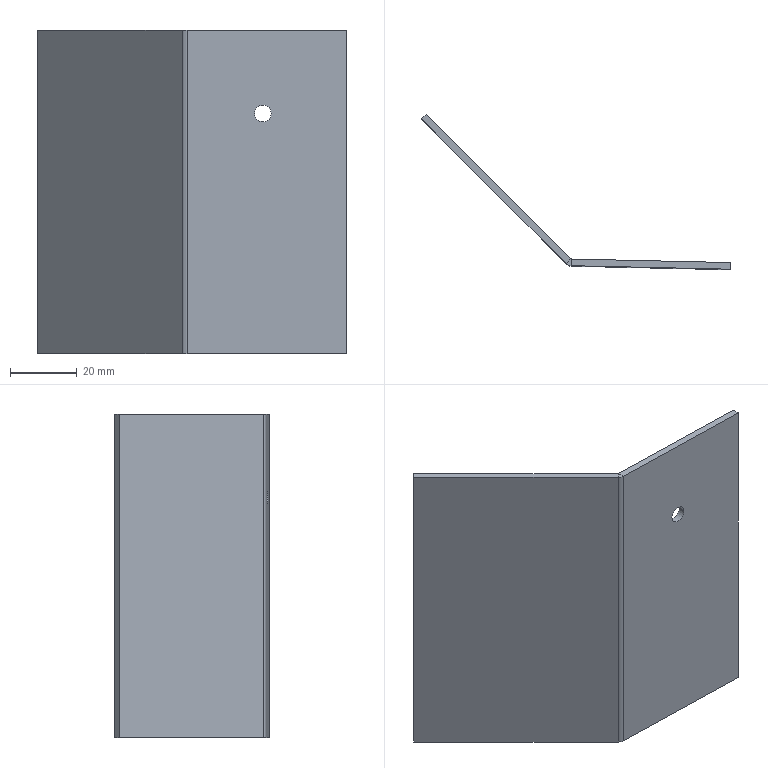Part | STEP file | Assembly TS-001-02 | 1 solid | 16 faces | box 92.488 x 46.409 x 97 mm | volume 21261 mm3 | plane 12 | cylinder 4 | commonest cylinder face diameters 5 x2 0.4 x1 4.4 x1
STEP:
#1=CARTESIAN_POINT('',(0.,0.,0.));
#2=DIRECTION('',(0.,0.,1.));
#3=DIRECTION('',(1.,0.,0.));
#4=AXIS2_PLACEMENT_3D('',#1,#2,#3);
#5=CARTESIAN_POINT('',(208.284,163.46,72.));
#6=VERTEX_POINT('',#5);
#7=CARTESIAN_POINT('',(208.329,165.46,72.));
#8=VERTEX_POINT('',#7);
#9=CARTESIAN_POINT('',(208.107,155.462,72.));
#10=DIRECTION('',(0.02216,0.9998,0.));
#11=VECTOR('',#10,1.);
#12=LINE('',#9,#11);
#13=CARTESIAN_POINT('',(210.607,155.407,72.));
#14=DIRECTION('',(0.02216,0.9998,0.));
#15=DIRECTION('',(-0.9998,0.02216,0.));
#16=AXIS2_PLACEMENT_3D('',#13,#14,#15);
#17=CYLINDRICAL_SURFACE('',#16,2.5);
#18=CARTESIAN_POINT('',(6.283,0.));
#19=DIRECTION('',(0.,1.));
#20=VECTOR('',#19,1.);
#21=LINE('',#18,#20);
#22=(GEOMETRIC_REPRESENTATION_CONTEXT(2)PARAMETRIC_REPRESENTATION_CONTEXT()REPRESENTATION_CONTEXT('',''));
#23=DEFINITIONAL_REPRESENTATION('',(#21),#22);
#24=PCURVE('',#17,#23);
#25=CARTESIAN_POINT('',(210.607,155.407,72.));
#26=DIRECTION('',(0.02216,0.9998,0.));
#27=DIRECTION('',(-0.9998,0.02216,0.));
#28=AXIS2_PLACEMENT_3D('',#25,#26,#27);
#29=CYLINDRICAL_SURFACE('',#28,2.5);
#30=CARTESIAN_POINT('',(0.,0.));
#31=DIRECTION('',(0.,1.));
#32=VECTOR('',#31,1.);
#33=LINE('',#30,#32);
#34=(GEOMETRIC_REPRESENTATION_CONTEXT(2)PARAMETRIC_REPRESENTATION_CONTEXT()REPRESENTATION_CONTEXT('',''));
#35=DEFINITIONAL_REPRESENTATION('',(#33),#34);
#36=PCURVE('',#29,#35);
#37=SURFACE_CURVE('',#12,(#24,#36),.PCURVE_S1.);
#38=EDGE_CURVE('',#6,#8,#37,.T.);
#39=ORIENTED_EDGE('',*,*,#38,.T.);
#40=CARTESIAN_POINT('',(213.328,165.349,72.));
#41=VERTEX_POINT('',#40);
#42=CARTESIAN_POINT('',(210.828,165.404,72.));
#43=DIRECTION('',(0.02216,0.9998,0.));
#44=DIRECTION('',(-0.9998,0.02216,0.));
#45=AXIS2_PLACEMENT_3D('',#42,#43,#44);
#46=CIRCLE('',#45,2.5);
#47=CARTESIAN_POINT('',(0.,10.));
#48=DIRECTION('',(1.,0.));
#49=VECTOR('',#48,1.);
#50=LINE('',#47,#49);
#51=(GEOMETRIC_REPRESENTATION_CONTEXT(2)PARAMETRIC_REPRESENTATION_CONTEXT()REPRESENTATION_CONTEXT('',''));
#52=DEFINITIONAL_REPRESENTATION('',(#50),#51);
#53=PCURVE('',#17,#52);
#54=CARTESIAN_POINT('',(242.32,164.706,97.));
#55=DIRECTION('',(-0.02216,-0.9998,0.));
#56=DIRECTION('',(0.9998,-0.02216,0.));
#57=AXIS2_PLACEMENT_3D('',#54,#55,#56);
#58=PLANE('',#57);
#59=CARTESIAN_POINT('',(-34.,-25.));
#60=CARTESIAN_POINT('',(-34.,-20.67));
#61=CARTESIAN_POINT('',(-30.25,-22.835));
#62=CARTESIAN_POINT('',(-26.5,-25.));
#63=CARTESIAN_POINT('',(-30.25,-27.165));
#64=CARTESIAN_POINT('',(-34.,-29.33));
#65=CARTESIAN_POINT('',(-34.,-25.));
#66=(BOUNDED_CURVE()B_SPLINE_CURVE(2,(#59,#60,#61,#62,#63,#64,#65),.UNSPECIFIED.,.T.,.F.)B_SPLINE_CURVE_WITH_KNOTS((1,2,2,2,2,1),(-2.094,0.,2.094,4.189,6.283,8.378),.UNSPECIFIED.)CURVE()GEOMETRIC_REPRESENTATION_ITEM()RATIONAL_B_SPLINE_CURVE((1.,0.5,1.,0.5,1.,0.5,1.))REPRESENTATION_ITEM(''));
#67=(GEOMETRIC_REPRESENTATION_CONTEXT(2)PARAMETRIC_REPRESENTATION_CONTEXT()REPRESENTATION_CONTEXT('',''));
#68=DEFINITIONAL_REPRESENTATION('',(#66),#67);
#69=PCURVE('',#58,#68);
#70=SURFACE_CURVE('',#46,(#53,#69),.PCURVE_S1.);
#71=EDGE_CURVE('',#41,#8,#70,.T.);
#72=ORIENTED_EDGE('',*,*,#71,.F.);
#73=CARTESIAN_POINT('',(213.283,163.349,72.));
#74=VERTEX_POINT('',#73);
#75=CARTESIAN_POINT('',(213.106,155.351,72.));
#76=DIRECTION('',(0.02216,0.9998,0.));
#77=VECTOR('',#76,1.);
#78=LINE('',#75,#77);
#79=CARTESIAN_POINT('',(3.142,0.));
#80=DIRECTION('',(0.,1.));
#81=VECTOR('',#80,1.);
#82=LINE('',#79,#81);
#83=(GEOMETRIC_REPRESENTATION_CONTEXT(2)PARAMETRIC_REPRESENTATION_CONTEXT()REPRESENTATION_CONTEXT('',''));
#84=DEFINITIONAL_REPRESENTATION('',(#82),#83);
#85=PCURVE('',#17,#84);
#86=CARTESIAN_POINT('',(3.142,0.));
#87=DIRECTION('',(0.,1.));
#88=VECTOR('',#87,1.);
#89=LINE('',#86,#88);
#90=(GEOMETRIC_REPRESENTATION_CONTEXT(2)PARAMETRIC_REPRESENTATION_CONTEXT()REPRESENTATION_CONTEXT('',''));
#91=DEFINITIONAL_REPRESENTATION('',(#89),#90);
#92=PCURVE('',#29,#91);
#93=SURFACE_CURVE('',#78,(#85,#92),.PCURVE_S1.);
#94=EDGE_CURVE('',#74,#41,#93,.T.);
#95=ORIENTED_EDGE('',*,*,#94,.F.);
#96=CARTESIAN_POINT('',(210.784,163.405,72.));
#97=DIRECTION('',(-0.02216,-0.9998,0.));
#98=DIRECTION('',(0.9998,-0.02216,0.));
#99=AXIS2_PLACEMENT_3D('',#96,#97,#98);
#100=CIRCLE('',#99,2.5);
#101=CARTESIAN_POINT('',(9.425,8.));
#102=DIRECTION('',(-1.,0.));
#103=VECTOR('',#102,1.);
#104=LINE('',#101,#103);
#105=(GEOMETRIC_REPRESENTATION_CONTEXT(2)PARAMETRIC_REPRESENTATION_CONTEXT()REPRESENTATION_CONTEXT('',''));
#106=DEFINITIONAL_REPRESENTATION('',(#104),#105);
#107=PCURVE('',#17,#106);
#108=CARTESIAN_POINT('',(242.276,162.707,97.));
#109=DIRECTION('',(-0.02216,-0.9998,0.));
#110=DIRECTION('',(0.9998,-0.02216,0.));
#111=AXIS2_PLACEMENT_3D('',#108,#109,#110);
#112=PLANE('',#111);
#113=CARTESIAN_POINT('',(-31.5,-25.));
#114=DIRECTION('',(1.,0.));
#115=AXIS2_PLACEMENT_2D('',#113,#114);
#116=CIRCLE('',#115,2.5);
#117=(GEOMETRIC_REPRESENTATION_CONTEXT(2)PARAMETRIC_REPRESENTATION_CONTEXT()REPRESENTATION_CONTEXT('',''));
#118=DEFINITIONAL_REPRESENTATION('',(#116),#117);
#119=PCURVE('',#112,#118);
#120=SURFACE_CURVE('',#100,(#107,#119),.PCURVE_S1.);
#121=EDGE_CURVE('',#6,#74,#120,.T.);
#122=ORIENTED_EDGE('',*,*,#121,.F.);
#123=EDGE_LOOP('',(#39,#72,#95,#122));
#124=FACE_BOUND('',#123,.F.);
#125=ADVANCED_FACE('',(#124),#17,.F.);
#126=CARTESIAN_POINT('',(186.63,164.551,97.));
#127=VERTEX_POINT('',#126);
#128=CARTESIAN_POINT('',(188.044,165.965,97.));
#129=VERTEX_POINT('',#128);
#130=CARTESIAN_POINT('',(186.63,164.551,97.));
#131=DIRECTION('',(0.7071,0.7071,0.));
#132=VECTOR('',#131,1.);
#133=LINE('',#130,#132);
#134=CARTESIAN_POINT('',(186.63,164.551,97.));
#135=DIRECTION('',(0.,0.,1.));
#136=DIRECTION('',(1.,0.,0.));
#137=AXIS2_PLACEMENT_3D('',#134,#135,#136);
#138=PLANE('',#137);
#139=CARTESIAN_POINT('',(0.,0.));
#140=DIRECTION('',(0.7071,0.7071));
#141=VECTOR('',#140,1.);
#142=LINE('',#139,#141);
#143=(GEOMETRIC_REPRESENTATION_CONTEXT(2)PARAMETRIC_REPRESENTATION_CONTEXT()REPRESENTATION_CONTEXT('',''));
#144=DEFINITIONAL_REPRESENTATION('',(#142),#143);
#145=PCURVE('',#138,#144);
#146=CARTESIAN_POINT('',(188.181,165.906,97.));
#147=DIRECTION('',(0.,0.,1.));
#148=DIRECTION('',(1.,0.,0.));
#149=AXIS2_PLACEMENT_3D('',#146,#147,#148);
#150=PLANE('',#149);
#151=CARTESIAN_POINT('',(-1.551,-1.356));
#152=DIRECTION('',(0.7071,0.7071));
#153=VECTOR('',#152,1.);
#154=LINE('',#151,#153);
#155=(GEOMETRIC_REPRESENTATION_CONTEXT(2)PARAMETRIC_REPRESENTATION_CONTEXT()REPRESENTATION_CONTEXT('',''));
#156=DEFINITIONAL_REPRESENTATION('',(#154),#155);
#157=PCURVE('',#150,#156);
#158=SURFACE_CURVE('',#133,(#145,#157),.PCURVE_S1.);
#159=EDGE_CURVE('',#127,#129,#158,.T.);
#160=ORIENTED_EDGE('',*,*,#159,.F.);
#161=CARTESIAN_POINT('',(188.136,163.907,97.));
#162=VERTEX_POINT('',#161);
#163=CARTESIAN_POINT('',(188.185,166.106,97.));
#164=DIRECTION('',(0.,0.,-1.));
#165=DIRECTION('',(1.,0.,0.));
#166=AXIS2_PLACEMENT_3D('',#163,#164,#165);
#167=CIRCLE('',#166,2.2);
#168=CARTESIAN_POINT('',(3.756,1.556));
#169=CARTESIAN_POINT('',(3.756,-2.255));
#170=CARTESIAN_POINT('',(0.4556,-0.3496));
#171=CARTESIAN_POINT('',(-2.844,1.556));
#172=CARTESIAN_POINT('',(0.4556,3.461));
#173=CARTESIAN_POINT('',(3.756,5.366));
#174=CARTESIAN_POINT('',(3.756,1.556));
#175=(BOUNDED_CURVE()B_SPLINE_CURVE(2,(#168,#169,#170,#171,#172,#173,#174),.UNSPECIFIED.,.T.,.F.)B_SPLINE_CURVE_WITH_KNOTS((1,2,2,2,2,1),(-2.094,0.,2.094,4.189,6.283,8.378),.UNSPECIFIED.)CURVE()GEOMETRIC_REPRESENTATION_ITEM()RATIONAL_B_SPLINE_CURVE((1.,0.5,1.,0.5,1.,0.5,1.))REPRESENTATION_ITEM(''));
#176=(GEOMETRIC_REPRESENTATION_CONTEXT(2)PARAMETRIC_REPRESENTATION_CONTEXT()REPRESENTATION_CONTEXT('',''));
#177=DEFINITIONAL_REPRESENTATION('',(#175),#176);
#178=PCURVE('',#138,#177);
#179=CARTESIAN_POINT('',(188.185,166.106,97.));
#180=DIRECTION('',(0.,0.,-1.));
#181=DIRECTION('',(-1.,0.,0.));
#182=AXIS2_PLACEMENT_3D('',#179,#180,#181);
#183=CYLINDRICAL_SURFACE('',#182,2.2);
#184=CARTESIAN_POINT('',(3.142,0.));
#185=DIRECTION('',(1.,0.));
#186=VECTOR('',#185,1.);
#187=LINE('',#184,#186);
#188=(GEOMETRIC_REPRESENTATION_CONTEXT(2)PARAMETRIC_REPRESENTATION_CONTEXT()REPRESENTATION_CONTEXT('',''));
#189=DEFINITIONAL_REPRESENTATION('',(#187),#188);
#190=PCURVE('',#183,#189);
#191=SURFACE_CURVE('',#167,(#178,#190),.PCURVE_S1.);
#192=EDGE_CURVE('',#162,#127,#191,.T.);
#193=ORIENTED_EDGE('',*,*,#192,.F.);
#194=CARTESIAN_POINT('',(188.181,165.906,97.));
#195=VERTEX_POINT('',#194);
#196=CARTESIAN_POINT('',(188.181,165.906,97.));
#197=DIRECTION('',(-0.02216,-0.9998,0.));
#198=VECTOR('',#197,1.);
#199=LINE('',#196,#198);
#200=CARTESIAN_POINT('',(1.551,1.356));
#201=DIRECTION('',(-0.02216,-0.9998));
#202=VECTOR('',#201,1.);
#203=LINE('',#200,#202);
#204=(GEOMETRIC_REPRESENTATION_CONTEXT(2)PARAMETRIC_REPRESENTATION_CONTEXT()REPRESENTATION_CONTEXT('',''));
#205=DEFINITIONAL_REPRESENTATION('',(#203),#204);
#206=PCURVE('',#138,#205);
#207=CARTESIAN_POINT('',(188.185,166.106,97.));
#208=DIRECTION('',(0.,0.,1.));
#209=DIRECTION('',(1.,0.,0.));
#210=AXIS2_PLACEMENT_3D('',#207,#208,#209);
#211=PLANE('',#210);
#212=CARTESIAN_POINT('',(-0.004433,-0.2));
#213=DIRECTION('',(-0.02216,-0.9998));
#214=VECTOR('',#213,1.);
#215=LINE('',#212,#214);
#216=(GEOMETRIC_REPRESENTATION_CONTEXT(2)PARAMETRIC_REPRESENTATION_CONTEXT()REPRESENTATION_CONTEXT('',''));
#217=DEFINITIONAL_REPRESENTATION('',(#215),#216);
#218=PCURVE('',#211,#217);
#219=SURFACE_CURVE('',#199,(#206,#218),.PCURVE_S1.);
#220=EDGE_CURVE('',#195,#162,#219,.T.);
#221=ORIENTED_EDGE('',*,*,#220,.F.);
#222=CARTESIAN_POINT('',(188.185,166.106,97.));
#223=DIRECTION('',(0.,0.,-1.));
#224=DIRECTION('',(1.,0.,0.));
#225=AXIS2_PLACEMENT_3D('',#222,#223,#224);
#226=CIRCLE('',#225,0.2);
#227=CARTESIAN_POINT('',(1.756,1.556));
#228=CARTESIAN_POINT('',(1.756,1.209));
#229=CARTESIAN_POINT('',(1.456,1.382));
#230=CARTESIAN_POINT('',(1.156,1.556));
#231=CARTESIAN_POINT('',(1.456,1.729));
#232=CARTESIAN_POINT('',(1.756,1.902));
#233=CARTESIAN_POINT('',(1.756,1.556));
#234=(BOUNDED_CURVE()B_SPLINE_CURVE(2,(#227,#228,#229,#230,#231,#232,#233),.UNSPECIFIED.,.T.,.F.)B_SPLINE_CURVE_WITH_KNOTS((1,2,2,2,2,1),(-2.094,0.,2.094,4.189,6.283,8.378),.UNSPECIFIED.)CURVE()GEOMETRIC_REPRESENTATION_ITEM()RATIONAL_B_SPLINE_CURVE((1.,0.5,1.,0.5,1.,0.5,1.))REPRESENTATION_ITEM(''));
#235=(GEOMETRIC_REPRESENTATION_CONTEXT(2)PARAMETRIC_REPRESENTATION_CONTEXT()REPRESENTATION_CONTEXT('',''));
#236=DEFINITIONAL_REPRESENTATION('',(#234),#235);
#237=PCURVE('',#138,#236);
#238=CARTESIAN_POINT('',(188.185,166.106,97.));
#239=DIRECTION('',(0.,0.,-1.));
#240=DIRECTION('',(-1.,0.,0.));
#241=AXIS2_PLACEMENT_3D('',#238,#239,#240);
#242=CYLINDRICAL_SURFACE('',#241,0.2);
#243=CARTESIAN_POINT('',(3.142,0.));
#244=DIRECTION('',(1.,0.));
#245=VECTOR('',#244,1.);
#246=LINE('',#243,#245);
#247=(GEOMETRIC_REPRESENTATION_CONTEXT(2)PARAMETRIC_REPRESENTATION_CONTEXT()REPRESENTATION_CONTEXT('',''));
#248=DEFINITIONAL_REPRESENTATION('',(#246),#247);
#249=PCURVE('',#242,#248);
#250=SURFACE_CURVE('',#226,(#237,#249),.PCURVE_S1.);
#251=EDGE_CURVE('',#195,#129,#250,.T.);
#252=ORIENTED_EDGE('',*,*,#251,.T.);
#253=EDGE_LOOP('',(#160,#193,#221,#252));
#254=FACE_BOUND('',#253,.T.);
#255=ADVANCED_FACE('',(#254),#138,.T.);
#256=CARTESIAN_POINT('',(143.335,207.846,97.));
#257=VERTEX_POINT('',#256);
#258=CARTESIAN_POINT('',(187.254,163.927,97.));
#259=DIRECTION('',(-0.7071,0.7071,0.));
#260=VECTOR('',#259,1.);
#261=LINE('',#258,#260);
#262=CARTESIAN_POINT('',(-0.9269,-1.98));
#263=DIRECTION('',(-0.7071,0.7071));
#264=VECTOR('',#263,1.);
#265=LINE('',#262,#264);
#266=(GEOMETRIC_REPRESENTATION_CONTEXT(2)PARAMETRIC_REPRESENTATION_CONTEXT()REPRESENTATION_CONTEXT('',''));
#267=DEFINITIONAL_REPRESENTATION('',(#265),#266);
#268=PCURVE('',#150,#267);
#269=CARTESIAN_POINT('',(187.254,163.927,97.));
#270=DIRECTION('',(-0.7071,-0.7071,0.));
#271=DIRECTION('',(0.7071,-0.7071,0.));
#272=AXIS2_PLACEMENT_3D('',#269,#270,#271);
#273=PLANE('',#272);
#274=CARTESIAN_POINT('',(0.,0.));
#275=DIRECTION('',(-1.,0.));
#276=VECTOR('',#275,1.);
#277=LINE('',#274,#276);
#278=(GEOMETRIC_REPRESENTATION_CONTEXT(2)PARAMETRIC_REPRESENTATION_CONTEXT()REPRESENTATION_CONTEXT('',''));
#279=DEFINITIONAL_REPRESENTATION('',(#277),#278);
#280=PCURVE('',#273,#279);
#281=SURFACE_CURVE('',#261,(#268,#280),.PCURVE_S1.);
#282=EDGE_CURVE('',#127,#257,#281,.T.);
#283=ORIENTED_EDGE('',*,*,#282,.F.);
#284=ORIENTED_EDGE('',*,*,#159,.T.);
#285=CARTESIAN_POINT('',(144.749,209.26,97.));
#286=VERTEX_POINT('',#285);
#287=CARTESIAN_POINT('',(188.668,165.341,97.));
#288=DIRECTION('',(-0.7071,0.7071,0.));
#289=VECTOR('',#288,1.);
#290=LINE('',#287,#289);
#291=CARTESIAN_POINT('',(0.4873,-0.5657));
#292=DIRECTION('',(-0.7071,0.7071));
#293=VECTOR('',#292,1.);
#294=LINE('',#291,#293);
#295=(GEOMETRIC_REPRESENTATION_CONTEXT(2)PARAMETRIC_REPRESENTATION_CONTEXT()REPRESENTATION_CONTEXT('',''));
#296=DEFINITIONAL_REPRESENTATION('',(#294),#295);
#297=PCURVE('',#150,#296);
#298=CARTESIAN_POINT('',(188.668,165.341,97.));
#299=DIRECTION('',(-0.7071,-0.7071,0.));
#300=DIRECTION('',(0.7071,-0.7071,0.));
#301=AXIS2_PLACEMENT_3D('',#298,#299,#300);
#302=PLANE('',#301);
#303=CARTESIAN_POINT('',(0.,0.));
#304=DIRECTION('',(-1.,0.));
#305=VECTOR('',#304,1.);
#306=LINE('',#303,#305);
#307=(GEOMETRIC_REPRESENTATION_CONTEXT(2)PARAMETRIC_REPRESENTATION_CONTEXT()REPRESENTATION_CONTEXT('',''));
#308=DEFINITIONAL_REPRESENTATION('',(#306),#307);
#309=PCURVE('',#302,#308);
#310=SURFACE_CURVE('',#290,(#297,#309),.PCURVE_S1.);
#311=EDGE_CURVE('',#129,#286,#310,.T.);
#312=ORIENTED_EDGE('',*,*,#311,.T.);
#313=CARTESIAN_POINT('',(143.335,207.846,97.));
#314=DIRECTION('',(0.7071,0.7071,0.));
#315=VECTOR('',#314,1.);
#316=LINE('',#313,#315);
#317=CARTESIAN_POINT('',(-44.846,41.939));
#318=DIRECTION('',(0.7071,0.7071));
#319=VECTOR('',#318,1.);
#320=LINE('',#317,#319);
#321=(GEOMETRIC_REPRESENTATION_CONTEXT(2)PARAMETRIC_REPRESENTATION_CONTEXT()REPRESENTATION_CONTEXT('',''));
#322=DEFINITIONAL_REPRESENTATION('',(#320),#321);
#323=PCURVE('',#150,#322);
#324=CARTESIAN_POINT('',(143.335,207.846,97.));
#325=DIRECTION('',(-0.7071,0.7071,0.));
#326=DIRECTION('',(-0.7071,-0.7071,0.));
#327=AXIS2_PLACEMENT_3D('',#324,#325,#326);
#328=PLANE('',#327);
#329=CARTESIAN_POINT('',(0.,0.));
#330=DIRECTION('',(-1.,0.));
#331=VECTOR('',#330,1.);
#332=LINE('',#329,#331);
#333=(GEOMETRIC_REPRESENTATION_CONTEXT(2)PARAMETRIC_REPRESENTATION_CONTEXT()REPRESENTATION_CONTEXT('',''));
#334=DEFINITIONAL_REPRESENTATION('',(#332),#333);
#335=PCURVE('',#328,#334);
#336=SURFACE_CURVE('',#316,(#323,#335),.PCURVE_S1.);
#337=EDGE_CURVE('',#257,#286,#336,.T.);
#338=ORIENTED_EDGE('',*,*,#337,.F.);
#339=EDGE_LOOP('',(#283,#284,#312,#338));
#340=FACE_BOUND('',#339,.T.);
#341=ADVANCED_FACE('',(#340),#150,.T.);
#342=CARTESIAN_POINT('',(188.136,163.907,0.));
#343=VERTEX_POINT('',#342);
#344=CARTESIAN_POINT('',(188.181,165.906,0.));
#345=VERTEX_POINT('',#344);
#346=CARTESIAN_POINT('',(188.136,163.907,0.));
#347=DIRECTION('',(0.02216,0.9998,0.));
#348=VECTOR('',#347,1.);
#349=LINE('',#346,#348);
#350=CARTESIAN_POINT('',(188.136,163.907,0.));
#351=DIRECTION('',(0.,0.,-1.));
#352=DIRECTION('',(-1.,0.,0.));
#353=AXIS2_PLACEMENT_3D('',#350,#351,#352);
#354=PLANE('',#353);
#355=CARTESIAN_POINT('',(0.,0.));
#356=DIRECTION('',(-0.02216,0.9998));
#357=VECTOR('',#356,1.);
#358=LINE('',#355,#357);
#359=(GEOMETRIC_REPRESENTATION_CONTEXT(2)PARAMETRIC_REPRESENTATION_CONTEXT()REPRESENTATION_CONTEXT('',''));
#360=DEFINITIONAL_REPRESENTATION('',(#358),#359);
#361=PCURVE('',#354,#360);
#362=CARTESIAN_POINT('',(188.044,165.965,0.));
#363=DIRECTION('',(0.,0.,-1.));
#364=DIRECTION('',(-1.,0.,0.));
#365=AXIS2_PLACEMENT_3D('',#362,#363,#364);
#366=PLANE('',#365);
#367=CARTESIAN_POINT('',(-0.09266,-2.058));
#368=DIRECTION('',(-0.02216,0.9998));
#369=VECTOR('',#368,1.);
#370=LINE('',#367,#369);
#371=(GEOMETRIC_REPRESENTATION_CONTEXT(2)PARAMETRIC_REPRESENTATION_CONTEXT()REPRESENTATION_CONTEXT('',''));
#372=DEFINITIONAL_REPRESENTATION('',(#370),#371);
#373=PCURVE('',#366,#372);
#374=SURFACE_CURVE('',#349,(#361,#373),.PCURVE_S1.);
#375=EDGE_CURVE('',#343,#345,#374,.T.);
#376=ORIENTED_EDGE('',*,*,#375,.F.);
#377=CARTESIAN_POINT('',(186.63,164.551,0.));
#378=VERTEX_POINT('',#377);
#379=CARTESIAN_POINT('',(188.185,166.106,0.));
#380=DIRECTION('',(0.,0.,-1.));
#381=DIRECTION('',(1.,0.,0.));
#382=AXIS2_PLACEMENT_3D('',#379,#380,#381);
#383=CIRCLE('',#382,2.2);
#384=CARTESIAN_POINT('',(-0.04876,2.199));
#385=DIRECTION('',(-1.,0.));
#386=AXIS2_PLACEMENT_2D('',#384,#385);
#387=CIRCLE('',#386,2.2);
#388=(GEOMETRIC_REPRESENTATION_CONTEXT(2)PARAMETRIC_REPRESENTATION_CONTEXT()REPRESENTATION_CONTEXT('',''));
#389=DEFINITIONAL_REPRESENTATION('',(#387),#388);
#390=PCURVE('',#354,#389);
#391=CARTESIAN_POINT('',(3.142,97.));
#392=DIRECTION('',(1.,0.));
#393=VECTOR('',#392,1.);
#394=LINE('',#391,#393);
#395=(GEOMETRIC_REPRESENTATION_CONTEXT(2)PARAMETRIC_REPRESENTATION_CONTEXT()REPRESENTATION_CONTEXT('',''));
#396=DEFINITIONAL_REPRESENTATION('',(#394),#395);
#397=PCURVE('',#183,#396);
#398=SURFACE_CURVE('',#383,(#390,#397),.PCURVE_S1.);
#399=EDGE_CURVE('',#343,#378,#398,.T.);
#400=ORIENTED_EDGE('',*,*,#399,.T.);
#401=CARTESIAN_POINT('',(188.044,165.965,0.));
#402=VERTEX_POINT('',#401);
#403=CARTESIAN_POINT('',(188.044,165.965,0.));
#404=DIRECTION('',(-0.7071,-0.7071,0.));
#405=VECTOR('',#404,1.);
#406=LINE('',#403,#405);
#407=CARTESIAN_POINT('',(0.09266,2.058));
#408=DIRECTION('',(0.7071,-0.7071));
#409=VECTOR('',#408,1.);
#410=LINE('',#407,#409);
#411=(GEOMETRIC_REPRESENTATION_CONTEXT(2)PARAMETRIC_REPRESENTATION_CONTEXT()REPRESENTATION_CONTEXT('',''));
#412=DEFINITIONAL_REPRESENTATION('',(#410),#411);
#413=PCURVE('',#354,#412);
#414=CARTESIAN_POINT('',(188.185,166.106,0.));
#415=DIRECTION('',(0.,0.,1.));
#416=DIRECTION('',(1.,0.,0.));
#417=AXIS2_PLACEMENT_3D('',#414,#415,#416);
#418=PLANE('',#417);
#419=CARTESIAN_POINT('',(-0.1414,-0.1414));
#420=DIRECTION('',(-0.7071,-0.7071));
#421=VECTOR('',#420,1.);
#422=LINE('',#419,#421);
#423=(GEOMETRIC_REPRESENTATION_CONTEXT(2)PARAMETRIC_REPRESENTATION_CONTEXT()REPRESENTATION_CONTEXT('',''));
#424=DEFINITIONAL_REPRESENTATION('',(#422),#423);
#425=PCURVE('',#418,#424);
#426=SURFACE_CURVE('',#406,(#413,#425),.PCURVE_S1.);
#427=EDGE_CURVE('',#402,#378,#426,.T.);
#428=ORIENTED_EDGE('',*,*,#427,.F.);
#429=CARTESIAN_POINT('',(188.185,166.106,0.));
#430=DIRECTION('',(0.,0.,-1.));
#431=DIRECTION('',(1.,0.,0.));
#432=AXIS2_PLACEMENT_3D('',#429,#430,#431);
#433=CIRCLE('',#432,0.2);
#434=CARTESIAN_POINT('',(-0.04876,2.199));
#435=DIRECTION('',(-1.,0.));
#436=AXIS2_PLACEMENT_2D('',#434,#435);
#437=CIRCLE('',#436,0.2);
#438=(GEOMETRIC_REPRESENTATION_CONTEXT(2)PARAMETRIC_REPRESENTATION_CONTEXT()REPRESENTATION_CONTEXT('',''));
#439=DEFINITIONAL_REPRESENTATION('',(#437),#438);
#440=PCURVE('',#354,#439);
#441=CARTESIAN_POINT('',(3.142,97.));
#442=DIRECTION('',(1.,0.));
#443=VECTOR('',#442,1.);
#444=LINE('',#441,#443);
#445=(GEOMETRIC_REPRESENTATION_CONTEXT(2)PARAMETRIC_REPRESENTATION_CONTEXT()REPRESENTATION_CONTEXT('',''));
#446=DEFINITIONAL_REPRESENTATION('',(#444),#445);
#447=PCURVE('',#242,#446);
#448=SURFACE_CURVE('',#433,(#440,#447),.PCURVE_S1.);
#449=EDGE_CURVE('',#345,#402,#448,.T.);
#450=ORIENTED_EDGE('',*,*,#449,.F.);
#451=EDGE_LOOP('',(#376,#400,#428,#450));
#452=FACE_BOUND('',#451,.T.);
#453=ADVANCED_FACE('',(#452),#354,.T.);
#454=CARTESIAN_POINT('',(235.778,162.851,0.));
#455=VERTEX_POINT('',#454);
#456=CARTESIAN_POINT('',(242.276,162.707,0.));
#457=DIRECTION('',(-0.9998,0.02216,0.));
#458=VECTOR('',#457,1.);
#459=LINE('',#456,#458);
#460=CARTESIAN_POINT('',(-54.232,-3.258));
#461=DIRECTION('',(0.9998,0.02216));
#462=VECTOR('',#461,1.);
#463=LINE('',#460,#462);
#464=(GEOMETRIC_REPRESENTATION_CONTEXT(2)PARAMETRIC_REPRESENTATION_CONTEXT()REPRESENTATION_CONTEXT('',''));
#465=DEFINITIONAL_REPRESENTATION('',(#463),#464);
#466=PCURVE('',#366,#465);
#467=CARTESIAN_POINT('',(0.,-97.));
#468=DIRECTION('',(-1.,0.));
#469=VECTOR('',#468,1.);
#470=LINE('',#467,#469);
#471=(GEOMETRIC_REPRESENTATION_CONTEXT(2)PARAMETRIC_REPRESENTATION_CONTEXT()REPRESENTATION_CONTEXT('',''));
#472=DEFINITIONAL_REPRESENTATION('',(#470),#471);
#473=PCURVE('',#112,#472);
#474=SURFACE_CURVE('',#459,(#466,#473),.PCURVE_S1.);
#475=EDGE_CURVE('',#455,#343,#474,.T.);
#476=ORIENTED_EDGE('',*,*,#475,.T.);
#477=ORIENTED_EDGE('',*,*,#375,.T.);
#478=CARTESIAN_POINT('',(235.822,164.85,0.));
#479=VERTEX_POINT('',#478);
#480=CARTESIAN_POINT('',(242.32,164.706,0.));
#481=DIRECTION('',(-0.9998,0.02216,0.));
#482=VECTOR('',#481,1.);
#483=LINE('',#480,#482);
#484=CARTESIAN_POINT('',(-54.277,-1.259));
#485=DIRECTION('',(0.9998,0.02216));
#486=VECTOR('',#485,1.);
#487=LINE('',#484,#486);
#488=(GEOMETRIC_REPRESENTATION_CONTEXT(2)PARAMETRIC_REPRESENTATION_CONTEXT()REPRESENTATION_CONTEXT('',''));
#489=DEFINITIONAL_REPRESENTATION('',(#487),#488);
#490=PCURVE('',#366,#489);
#491=CARTESIAN_POINT('',(0.,-97.));
#492=DIRECTION('',(-1.,0.));
#493=VECTOR('',#492,1.);
#494=LINE('',#491,#493);
#495=(GEOMETRIC_REPRESENTATION_CONTEXT(2)PARAMETRIC_REPRESENTATION_CONTEXT()REPRESENTATION_CONTEXT('',''));
#496=DEFINITIONAL_REPRESENTATION('',(#494),#495);
#497=PCURVE('',#58,#496);
#498=SURFACE_CURVE('',#483,(#490,#497),.PCURVE_S1.);
#499=EDGE_CURVE('',#479,#345,#498,.T.);
#500=ORIENTED_EDGE('',*,*,#499,.F.);
#501=CARTESIAN_POINT('',(235.823,164.906,0.));
#502=DIRECTION('',(-0.02216,-0.9998,0.));
#503=VECTOR('',#502,1.);
#504=LINE('',#501,#503);
#505=CARTESIAN_POINT('',(-47.78,-1.059));
#506=DIRECTION('',(0.02216,-0.9998));
#507=VECTOR('',#506,1.);
#508=LINE('',#505,#507);
#509=(GEOMETRIC_REPRESENTATION_CONTEXT(2)PARAMETRIC_REPRESENTATION_CONTEXT()REPRESENTATION_CONTEXT('',''));
#510=DEFINITIONAL_REPRESENTATION('',(#508),#509);
#511=PCURVE('',#366,#510);
#512=CARTESIAN_POINT('',(235.822,164.85,97.));
#513=DIRECTION('',(0.9998,-0.02216,0.));
#514=DIRECTION('',(0.02216,0.9998,0.));
#515=AXIS2_PLACEMENT_3D('',#512,#513,#514);
#516=PLANE('',#515);
#517=CARTESIAN_POINT('',(0.05548,-97.));
#518=DIRECTION('',(-1.,0.));
#519=VECTOR('',#518,1.);
#520=LINE('',#517,#519);
#521=(GEOMETRIC_REPRESENTATION_CONTEXT(2)PARAMETRIC_REPRESENTATION_CONTEXT()REPRESENTATION_CONTEXT('',''));
#522=DEFINITIONAL_REPRESENTATION('',(#520),#521);
#523=PCURVE('',#516,#522);
#524=SURFACE_CURVE('',#504,(#511,#523),.PCURVE_S1.);
#525=EDGE_CURVE('',#479,#455,#524,.T.);
#526=ORIENTED_EDGE('',*,*,#525,.T.);
#527=EDGE_LOOP('',(#476,#477,#500,#526));
#528=FACE_BOUND('',#527,.T.);
#529=ADVANCED_FACE('',(#528),#366,.T.);
#530=CARTESIAN_POINT('',(144.749,209.26,0.));
#531=VERTEX_POINT('',#530);
#532=CARTESIAN_POINT('',(188.668,165.341,0.));
#533=DIRECTION('',(-0.7071,0.7071,0.));
#534=VECTOR('',#533,1.);
#535=LINE('',#532,#534);
#536=CARTESIAN_POINT('',(0.,-97.));
#537=DIRECTION('',(-1.,0.));
#538=VECTOR('',#537,1.);
#539=LINE('',#536,#538);
#540=(GEOMETRIC_REPRESENTATION_CONTEXT(2)PARAMETRIC_REPRESENTATION_CONTEXT()REPRESENTATION_CONTEXT('',''));
#541=DEFINITIONAL_REPRESENTATION('',(#539),#540);
#542=PCURVE('',#302,#541);
#543=CARTESIAN_POINT('',(0.4828,-0.7657));
#544=DIRECTION('',(-0.7071,0.7071));
#545=VECTOR('',#544,1.);
#546=LINE('',#543,#545);
#547=(GEOMETRIC_REPRESENTATION_CONTEXT(2)PARAMETRIC_REPRESENTATION_CONTEXT()REPRESENTATION_CONTEXT('',''));
#548=DEFINITIONAL_REPRESENTATION('',(#546),#547);
#549=PCURVE('',#418,#548);
#550=SURFACE_CURVE('',#535,(#542,#549),.PCURVE_S1.);
#551=EDGE_CURVE('',#402,#531,#550,.T.);
#552=ORIENTED_EDGE('',*,*,#551,.T.);
#553=CARTESIAN_POINT('',(144.749,209.26,97.));
#554=DIRECTION('',(0.,0.,-1.));
#555=VECTOR('',#554,1.);
#556=LINE('',#553,#555);
#557=CARTESIAN_POINT('',(-62.111,0.));
#558=DIRECTION('',(0.,-1.));
#559=VECTOR('',#558,1.);
#560=LINE('',#557,#559);
#561=(GEOMETRIC_REPRESENTATION_CONTEXT(2)PARAMETRIC_REPRESENTATION_CONTEXT()REPRESENTATION_CONTEXT('',''));
#562=DEFINITIONAL_REPRESENTATION('',(#560),#561);
#563=PCURVE('',#302,#562);
#564=CARTESIAN_POINT('',(-2.,0.));
#565=DIRECTION('',(0.,-1.));
#566=VECTOR('',#565,1.);
#567=LINE('',#564,#566);
#568=(GEOMETRIC_REPRESENTATION_CONTEXT(2)PARAMETRIC_REPRESENTATION_CONTEXT()REPRESENTATION_CONTEXT('',''));
#569=DEFINITIONAL_REPRESENTATION('',(#567),#568);
#570=PCURVE('',#328,#569);
#571=SURFACE_CURVE('',#556,(#563,#570),.PCURVE_S1.);
#572=EDGE_CURVE('',#286,#531,#571,.T.);
#573=ORIENTED_EDGE('',*,*,#572,.F.);
#574=ORIENTED_EDGE('',*,*,#311,.F.);
#575=CARTESIAN_POINT('',(188.044,165.965,97.));
#576=DIRECTION('',(0.,0.,-1.));
#577=VECTOR('',#576,1.);
#578=LINE('',#575,#577);
#579=CARTESIAN_POINT('',(-0.8828,0.));
#580=DIRECTION('',(0.,-1.));
#581=VECTOR('',#580,1.);
#582=LINE('',#579,#581);
#583=(GEOMETRIC_REPRESENTATION_CONTEXT(2)PARAMETRIC_REPRESENTATION_CONTEXT()REPRESENTATION_CONTEXT('',''));
#584=DEFINITIONAL_REPRESENTATION('',(#582),#583);
#585=PCURVE('',#302,#584);
#586=CARTESIAN_POINT('',(5.498,0.));
#587=DIRECTION('',(0.,1.));
#588=VECTOR('',#587,1.);
#589=LINE('',#586,#588);
#590=(GEOMETRIC_REPRESENTATION_CONTEXT(2)PARAMETRIC_REPRESENTATION_CONTEXT()REPRESENTATION_CONTEXT('',''));
#591=DEFINITIONAL_REPRESENTATION('',(#589),#590);
#592=PCURVE('',#242,#591);
#593=SURFACE_CURVE('',#578,(#585,#592),.PCURVE_S1.);
#594=EDGE_CURVE('',#129,#402,#593,.T.);
#595=ORIENTED_EDGE('',*,*,#594,.T.);
#596=EDGE_LOOP('',(#552,#573,#574,#595));
#597=FACE_BOUND('',#596,.T.);
#598=ADVANCED_FACE('',(#597),#302,.F.);
#599=CARTESIAN_POINT('',(143.335,207.846,0.));
#600=VERTEX_POINT('',#599);
#601=CARTESIAN_POINT('',(143.335,207.846,0.));
#602=DIRECTION('',(0.7071,0.7071,0.));
#603=VECTOR('',#602,1.);
#604=LINE('',#601,#603);
#605=CARTESIAN_POINT('',(0.,-97.));
#606=DIRECTION('',(-1.,0.));
#607=VECTOR('',#606,1.);
#608=LINE('',#605,#607);
#609=(GEOMETRIC_REPRESENTATION_CONTEXT(2)PARAMETRIC_REPRESENTATION_CONTEXT()REPRESENTATION_CONTEXT('',''));
#610=DEFINITIONAL_REPRESENTATION('',(#608),#609);
#611=PCURVE('',#328,#610);
#612=CARTESIAN_POINT('',(-44.851,41.739));
#613=DIRECTION('',(0.7071,0.7071));
#614=VECTOR('',#613,1.);
#615=LINE('',#612,#614);
#616=(GEOMETRIC_REPRESENTATION_CONTEXT(2)PARAMETRIC_REPRESENTATION_CONTEXT()REPRESENTATION_CONTEXT('',''));
#617=DEFINITIONAL_REPRESENTATION('',(#615),#616);
#618=PCURVE('',#418,#617);
#619=SURFACE_CURVE('',#604,(#611,#618),.PCURVE_S1.);
#620=EDGE_CURVE('',#600,#531,#619,.T.);
#621=ORIENTED_EDGE('',*,*,#620,.F.);
#622=CARTESIAN_POINT('',(143.335,207.846,97.));
#623=DIRECTION('',(0.,0.,-1.));
#624=VECTOR('',#623,1.);
#625=LINE('',#622,#624);
#626=CARTESIAN_POINT('',(0.,0.));
#627=DIRECTION('',(0.,-1.));
#628=VECTOR('',#627,1.);
#629=LINE('',#626,#628);
#630=(GEOMETRIC_REPRESENTATION_CONTEXT(2)PARAMETRIC_REPRESENTATION_CONTEXT()REPRESENTATION_CONTEXT('',''));
#631=DEFINITIONAL_REPRESENTATION('',(#629),#630);
#632=PCURVE('',#328,#631);
#633=CARTESIAN_POINT('',(-62.111,0.));
#634=DIRECTION('',(0.,-1.));
#635=VECTOR('',#634,1.);
#636=LINE('',#633,#635);
#637=(GEOMETRIC_REPRESENTATION_CONTEXT(2)PARAMETRIC_REPRESENTATION_CONTEXT()REPRESENTATION_CONTEXT('',''));
#638=DEFINITIONAL_REPRESENTATION('',(#636),#637);
#639=PCURVE('',#273,#638);
#640=SURFACE_CURVE('',#625,(#632,#639),.PCURVE_S1.);
#641=EDGE_CURVE('',#257,#600,#640,.T.);
#642=ORIENTED_EDGE('',*,*,#641,.F.);
#643=ORIENTED_EDGE('',*,*,#337,.T.);
#644=ORIENTED_EDGE('',*,*,#572,.T.);
#645=EDGE_LOOP('',(#621,#642,#643,#644));
#646=FACE_BOUND('',#645,.T.);
#647=ADVANCED_FACE('',(#646),#328,.T.);
#648=CARTESIAN_POINT('',(187.254,163.927,0.));
#649=DIRECTION('',(-0.7071,0.7071,0.));
#650=VECTOR('',#649,1.);
#651=LINE('',#648,#650);
#652=CARTESIAN_POINT('',(0.,-97.));
#653=DIRECTION('',(-1.,0.));
#654=VECTOR('',#653,1.);
#655=LINE('',#652,#654);
#656=(GEOMETRIC_REPRESENTATION_CONTEXT(2)PARAMETRIC_REPRESENTATION_CONTEXT()REPRESENTATION_CONTEXT('',''));
#657=DEFINITIONAL_REPRESENTATION('',(#655),#656);
#658=PCURVE('',#273,#657);
#659=CARTESIAN_POINT('',(-0.9314,-2.18));
#660=DIRECTION('',(-0.7071,0.7071));
#661=VECTOR('',#660,1.);
#662=LINE('',#659,#661);
#663=(GEOMETRIC_REPRESENTATION_CONTEXT(2)PARAMETRIC_REPRESENTATION_CONTEXT()REPRESENTATION_CONTEXT('',''));
#664=DEFINITIONAL_REPRESENTATION('',(#662),#663);
#665=PCURVE('',#418,#664);
#666=SURFACE_CURVE('',#651,(#658,#665),.PCURVE_S1.);
#667=EDGE_CURVE('',#378,#600,#666,.T.);
#668=ORIENTED_EDGE('',*,*,#667,.F.);
#669=CARTESIAN_POINT('',(186.63,164.551,97.));
#670=DIRECTION('',(0.,0.,-1.));
#671=VECTOR('',#670,1.);
#672=LINE('',#669,#671);
#673=CARTESIAN_POINT('',(-0.8828,0.));
#674=DIRECTION('',(0.,-1.));
#675=VECTOR('',#674,1.);
#676=LINE('',#673,#675);
#677=(GEOMETRIC_REPRESENTATION_CONTEXT(2)PARAMETRIC_REPRESENTATION_CONTEXT()REPRESENTATION_CONTEXT('',''));
#678=DEFINITIONAL_REPRESENTATION('',(#676),#677);
#679=PCURVE('',#273,#678);
#680=CARTESIAN_POINT('',(5.498,0.));
#681=DIRECTION('',(0.,1.));
#682=VECTOR('',#681,1.);
#683=LINE('',#680,#682);
#684=(GEOMETRIC_REPRESENTATION_CONTEXT(2)PARAMETRIC_REPRESENTATION_CONTEXT()REPRESENTATION_CONTEXT('',''));
#685=DEFINITIONAL_REPRESENTATION('',(#683),#684);
#686=PCURVE('',#183,#685);
#687=SURFACE_CURVE('',#672,(#679,#686),.PCURVE_S1.);
#688=EDGE_CURVE('',#127,#378,#687,.T.);
#689=ORIENTED_EDGE('',*,*,#688,.F.);
#690=ORIENTED_EDGE('',*,*,#282,.T.);
#691=ORIENTED_EDGE('',*,*,#641,.T.);
#692=EDGE_LOOP('',(#668,#689,#690,#691));
#693=FACE_BOUND('',#692,.T.);
#694=ADVANCED_FACE('',(#693),#273,.T.);
#695=ORIENTED_EDGE('',*,*,#399,.F.);
#696=CARTESIAN_POINT('',(188.136,163.907,97.));
#697=DIRECTION('',(0.,0.,-1.));
#698=VECTOR('',#697,1.);
#699=LINE('',#696,#698);
#700=CARTESIAN_POINT('',(4.735,0.));
#701=DIRECTION('',(0.,1.));
#702=VECTOR('',#701,1.);
#703=LINE('',#700,#702);
#704=(GEOMETRIC_REPRESENTATION_CONTEXT(2)PARAMETRIC_REPRESENTATION_CONTEXT()REPRESENTATION_CONTEXT('',''));
#705=DEFINITIONAL_REPRESENTATION('',(#703),#704);
#706=PCURVE('',#183,#705);
#707=CARTESIAN_POINT('',(-54.153,0.));
#708=DIRECTION('',(0.,-1.));
#709=VECTOR('',#708,1.);
#710=LINE('',#707,#709);
#711=(GEOMETRIC_REPRESENTATION_CONTEXT(2)PARAMETRIC_REPRESENTATION_CONTEXT()REPRESENTATION_CONTEXT('',''));
#712=DEFINITIONAL_REPRESENTATION('',(#710),#711);
#713=PCURVE('',#112,#712);
#714=SURFACE_CURVE('',#699,(#706,#713),.PCURVE_S1.);
#715=EDGE_CURVE('',#162,#343,#714,.T.);
#716=ORIENTED_EDGE('',*,*,#715,.F.);
#717=ORIENTED_EDGE('',*,*,#192,.T.);
#718=ORIENTED_EDGE('',*,*,#688,.T.);
#719=EDGE_LOOP('',(#695,#716,#717,#718));
#720=FACE_BOUND('',#719,.T.);
#721=ADVANCED_FACE('',(#720),#183,.T.);
#722=ORIENTED_EDGE('',*,*,#121,.F.);
#723=CARTESIAN_POINT('',(210.784,163.405,72.));
#724=DIRECTION('',(-0.02216,-0.9998,0.));
#725=DIRECTION('',(0.9998,-0.02216,0.));
#726=AXIS2_PLACEMENT_3D('',#723,#724,#725);
#727=CIRCLE('',#726,2.5);
#728=CARTESIAN_POINT('',(-31.5,-25.));
#729=DIRECTION('',(1.,0.));
#730=AXIS2_PLACEMENT_2D('',#728,#729);
#731=CIRCLE('',#730,2.5);
#732=(GEOMETRIC_REPRESENTATION_CONTEXT(2)PARAMETRIC_REPRESENTATION_CONTEXT()REPRESENTATION_CONTEXT('',''));
#733=DEFINITIONAL_REPRESENTATION('',(#731),#732);
#734=PCURVE('',#112,#733);
#735=CARTESIAN_POINT('',(3.142,8.));
#736=DIRECTION('',(-1.,0.));
#737=VECTOR('',#736,1.);
#738=LINE('',#735,#737);
#739=(GEOMETRIC_REPRESENTATION_CONTEXT(2)PARAMETRIC_REPRESENTATION_CONTEXT()REPRESENTATION_CONTEXT('',''));
#740=DEFINITIONAL_REPRESENTATION('',(#738),#739);
#741=PCURVE('',#29,#740);
#742=SURFACE_CURVE('',#727,(#734,#741),.PCURVE_S1.);
#743=EDGE_CURVE('',#74,#6,#742,.T.);
#744=ORIENTED_EDGE('',*,*,#743,.F.);
#745=EDGE_LOOP('',(#722,#744));
#746=FACE_BOUND('',#745,.T.);
#747=ORIENTED_EDGE('',*,*,#475,.F.);
#748=CARTESIAN_POINT('',(235.778,162.851,97.));
#749=VERTEX_POINT('',#748);
#750=CARTESIAN_POINT('',(235.778,162.851,97.));
#751=DIRECTION('',(0.,0.,-1.));
#752=VECTOR('',#751,1.);
#753=LINE('',#750,#752);
#754=CARTESIAN_POINT('',(-6.5,0.));
#755=DIRECTION('',(0.,-1.));
#756=VECTOR('',#755,1.);
#757=LINE('',#754,#756);
#758=(GEOMETRIC_REPRESENTATION_CONTEXT(2)PARAMETRIC_REPRESENTATION_CONTEXT()REPRESENTATION_CONTEXT('',''));
#759=DEFINITIONAL_REPRESENTATION('',(#757),#758);
#760=PCURVE('',#112,#759);
#761=CARTESIAN_POINT('',(-2.,0.));
#762=DIRECTION('',(0.,-1.));
#763=VECTOR('',#762,1.);
#764=LINE('',#761,#763);
#765=(GEOMETRIC_REPRESENTATION_CONTEXT(2)PARAMETRIC_REPRESENTATION_CONTEXT()REPRESENTATION_CONTEXT('',''));
#766=DEFINITIONAL_REPRESENTATION('',(#764),#765);
#767=PCURVE('',#516,#766);
#768=SURFACE_CURVE('',#753,(#760,#767),.PCURVE_S1.);
#769=EDGE_CURVE('',#749,#455,#768,.T.);
#770=ORIENTED_EDGE('',*,*,#769,.F.);
#771=CARTESIAN_POINT('',(242.276,162.707,97.));
#772=DIRECTION('',(-0.9998,0.02216,0.));
#773=VECTOR('',#772,1.);
#774=LINE('',#771,#773);
#775=CARTESIAN_POINT('',(0.,0.));
#776=DIRECTION('',(-1.,0.));
#777=VECTOR('',#776,1.);
#778=LINE('',#775,#777);
#779=(GEOMETRIC_REPRESENTATION_CONTEXT(2)PARAMETRIC_REPRESENTATION_CONTEXT()REPRESENTATION_CONTEXT('',''));
#780=DEFINITIONAL_REPRESENTATION('',(#778),#779);
#781=PCURVE('',#112,#780);
#782=CARTESIAN_POINT('',(54.091,-3.4));
#783=DIRECTION('',(-0.9998,0.02216));
#784=VECTOR('',#783,1.);
#785=LINE('',#782,#784);
#786=(GEOMETRIC_REPRESENTATION_CONTEXT(2)PARAMETRIC_REPRESENTATION_CONTEXT()REPRESENTATION_CONTEXT('',''));
#787=DEFINITIONAL_REPRESENTATION('',(#785),#786);
#788=PCURVE('',#211,#787);
#789=SURFACE_CURVE('',#774,(#781,#788),.PCURVE_S1.);
#790=EDGE_CURVE('',#749,#162,#789,.T.);
#791=ORIENTED_EDGE('',*,*,#790,.T.);
#792=ORIENTED_EDGE('',*,*,#715,.T.);
#793=EDGE_LOOP('',(#747,#770,#791,#792));
#794=FACE_BOUND('',#793,.T.);
#795=ADVANCED_FACE('',(#746,#794),#112,.T.);
#796=ORIENTED_EDGE('',*,*,#525,.F.);
#797=CARTESIAN_POINT('',(235.822,164.85,97.));
#798=VERTEX_POINT('',#797);
#799=CARTESIAN_POINT('',(235.822,164.85,97.));
#800=DIRECTION('',(0.,0.,-1.));
#801=VECTOR('',#800,1.);
#802=LINE('',#799,#801);
#803=CARTESIAN_POINT('',(0.,0.));
#804=DIRECTION('',(0.,-1.));
#805=VECTOR('',#804,1.);
#806=LINE('',#803,#805);
#807=(GEOMETRIC_REPRESENTATION_CONTEXT(2)PARAMETRIC_REPRESENTATION_CONTEXT()REPRESENTATION_CONTEXT('',''));
#808=DEFINITIONAL_REPRESENTATION('',(#806),#807);
#809=PCURVE('',#516,#808);
#810=CARTESIAN_POINT('',(-6.5,0.));
#811=DIRECTION('',(0.,-1.));
#812=VECTOR('',#811,1.);
#813=LINE('',#810,#812);
#814=(GEOMETRIC_REPRESENTATION_CONTEXT(2)PARAMETRIC_REPRESENTATION_CONTEXT()REPRESENTATION_CONTEXT('',''));
#815=DEFINITIONAL_REPRESENTATION('',(#813),#814);
#816=PCURVE('',#58,#815);
#817=SURFACE_CURVE('',#802,(#809,#816),.PCURVE_S1.);
#818=EDGE_CURVE('',#798,#479,#817,.T.);
#819=ORIENTED_EDGE('',*,*,#818,.F.);
#820=CARTESIAN_POINT('',(235.822,164.85,97.));
#821=DIRECTION('',(-0.02216,-0.9998,0.));
#822=VECTOR('',#821,1.);
#823=LINE('',#820,#822);
#824=CARTESIAN_POINT('',(0.,0.));
#825=DIRECTION('',(-1.,0.));
#826=VECTOR('',#825,1.);
#827=LINE('',#824,#826);
#828=(GEOMETRIC_REPRESENTATION_CONTEXT(2)PARAMETRIC_REPRESENTATION_CONTEXT()REPRESENTATION_CONTEXT('',''));
#829=DEFINITIONAL_REPRESENTATION('',(#827),#828);
#830=PCURVE('',#516,#829);
#831=CARTESIAN_POINT('',(47.637,-1.256));
#832=DIRECTION('',(-0.02216,-0.9998));
#833=VECTOR('',#832,1.);
#834=LINE('',#831,#833);
#835=(GEOMETRIC_REPRESENTATION_CONTEXT(2)PARAMETRIC_REPRESENTATION_CONTEXT()REPRESENTATION_CONTEXT('',''));
#836=DEFINITIONAL_REPRESENTATION('',(#834),#835);
#837=PCURVE('',#211,#836);
#838=SURFACE_CURVE('',#823,(#830,#837),.PCURVE_S1.);
#839=EDGE_CURVE('',#798,#749,#838,.T.);
#840=ORIENTED_EDGE('',*,*,#839,.T.);
#841=ORIENTED_EDGE('',*,*,#769,.T.);
#842=EDGE_LOOP('',(#796,#819,#840,#841));
#843=FACE_BOUND('',#842,.T.);
#844=ADVANCED_FACE('',(#843),#516,.T.);
#845=CARTESIAN_POINT('',(210.828,165.404,72.));
#846=DIRECTION('',(0.02216,0.9998,0.));
#847=DIRECTION('',(-0.9998,0.02216,0.));
#848=AXIS2_PLACEMENT_3D('',#845,#846,#847);
#849=CIRCLE('',#848,2.5);
#850=CARTESIAN_POINT('',(-34.,-25.));
#851=CARTESIAN_POINT('',(-34.,-20.67));
#852=CARTESIAN_POINT('',(-30.25,-22.835));
#853=CARTESIAN_POINT('',(-26.5,-25.));
#854=CARTESIAN_POINT('',(-30.25,-27.165));
#855=CARTESIAN_POINT('',(-34.,-29.33));
#856=CARTESIAN_POINT('',(-34.,-25.));
#857=(BOUNDED_CURVE()B_SPLINE_CURVE(2,(#850,#851,#852,#853,#854,#855,#856),.UNSPECIFIED.,.T.,.F.)B_SPLINE_CURVE_WITH_KNOTS((1,2,2,2,2,1),(-2.094,0.,2.094,4.189,6.283,8.378),.UNSPECIFIED.)CURVE()GEOMETRIC_REPRESENTATION_ITEM()RATIONAL_B_SPLINE_CURVE((1.,0.5,1.,0.5,1.,0.5,1.))REPRESENTATION_ITEM(''));
#858=(GEOMETRIC_REPRESENTATION_CONTEXT(2)PARAMETRIC_REPRESENTATION_CONTEXT()REPRESENTATION_CONTEXT('',''));
#859=DEFINITIONAL_REPRESENTATION('',(#857),#858);
#860=PCURVE('',#58,#859);
#861=CARTESIAN_POINT('',(0.,10.));
#862=DIRECTION('',(1.,0.));
#863=VECTOR('',#862,1.);
#864=LINE('',#861,#863);
#865=(GEOMETRIC_REPRESENTATION_CONTEXT(2)PARAMETRIC_REPRESENTATION_CONTEXT()REPRESENTATION_CONTEXT('',''));
#866=DEFINITIONAL_REPRESENTATION('',(#864),#865);
#867=PCURVE('',#29,#866);
#868=SURFACE_CURVE('',#849,(#860,#867),.PCURVE_S1.);
#869=EDGE_CURVE('',#8,#41,#868,.T.);
#870=ORIENTED_EDGE('',*,*,#869,.F.);
#871=ORIENTED_EDGE('',*,*,#71,.F.);
#872=EDGE_LOOP('',(#870,#871));
#873=FACE_BOUND('',#872,.T.);
#874=ORIENTED_EDGE('',*,*,#499,.T.);
#875=CARTESIAN_POINT('',(188.181,165.906,97.));
#876=DIRECTION('',(0.,0.,-1.));
#877=VECTOR('',#876,1.);
#878=LINE('',#875,#877);
#879=CARTESIAN_POINT('',(-54.153,0.));
#880=DIRECTION('',(0.,-1.));
#881=VECTOR('',#880,1.);
#882=LINE('',#879,#881);
#883=(GEOMETRIC_REPRESENTATION_CONTEXT(2)PARAMETRIC_REPRESENTATION_CONTEXT()REPRESENTATION_CONTEXT('',''));
#884=DEFINITIONAL_REPRESENTATION('',(#882),#883);
#885=PCURVE('',#58,#884);
#886=CARTESIAN_POINT('',(4.735,0.));
#887=DIRECTION('',(0.,1.));
#888=VECTOR('',#887,1.);
#889=LINE('',#886,#888);
#890=(GEOMETRIC_REPRESENTATION_CONTEXT(2)PARAMETRIC_REPRESENTATION_CONTEXT()REPRESENTATION_CONTEXT('',''));
#891=DEFINITIONAL_REPRESENTATION('',(#889),#890);
#892=PCURVE('',#242,#891);
#893=SURFACE_CURVE('',#878,(#885,#892),.PCURVE_S1.);
#894=EDGE_CURVE('',#195,#345,#893,.T.);
#895=ORIENTED_EDGE('',*,*,#894,.F.);
#896=CARTESIAN_POINT('',(242.32,164.706,97.));
#897=DIRECTION('',(-0.9998,0.02216,0.));
#898=VECTOR('',#897,1.);
#899=LINE('',#896,#898);
#900=CARTESIAN_POINT('',(0.,0.));
#901=DIRECTION('',(-1.,0.));
#902=VECTOR('',#901,1.);
#903=LINE('',#900,#902);
#904=(GEOMETRIC_REPRESENTATION_CONTEXT(2)PARAMETRIC_REPRESENTATION_CONTEXT()REPRESENTATION_CONTEXT('',''));
#905=DEFINITIONAL_REPRESENTATION('',(#903),#904);
#906=PCURVE('',#58,#905);
#907=CARTESIAN_POINT('',(54.135,-1.4));
#908=DIRECTION('',(-0.9998,0.02216));
#909=VECTOR('',#908,1.);
#910=LINE('',#907,#909);
#911=(GEOMETRIC_REPRESENTATION_CONTEXT(2)PARAMETRIC_REPRESENTATION_CONTEXT()REPRESENTATION_CONTEXT('',''));
#912=DEFINITIONAL_REPRESENTATION('',(#910),#911);
#913=PCURVE('',#211,#912);
#914=SURFACE_CURVE('',#899,(#906,#913),.PCURVE_S1.);
#915=EDGE_CURVE('',#798,#195,#914,.T.);
#916=ORIENTED_EDGE('',*,*,#915,.F.);
#917=ORIENTED_EDGE('',*,*,#818,.T.);
#918=EDGE_LOOP('',(#874,#895,#916,#917));
#919=FACE_BOUND('',#918,.T.);
#920=ADVANCED_FACE('',(#873,#919),#58,.F.);
#921=ORIENTED_EDGE('',*,*,#894,.F.);
#922=ORIENTED_EDGE('',*,*,#251,.T.);
#923=ORIENTED_EDGE('',*,*,#594,.T.);
#924=ORIENTED_EDGE('',*,*,#449,.F.);
#925=EDGE_LOOP('',(#921,#922,#923,#924));
#926=FACE_BOUND('',#925,.F.);
#927=ADVANCED_FACE('',(#926),#242,.F.);
#928=ORIENTED_EDGE('',*,*,#915,.T.);
#929=ORIENTED_EDGE('',*,*,#220,.T.);
#930=ORIENTED_EDGE('',*,*,#790,.F.);
#931=ORIENTED_EDGE('',*,*,#839,.F.);
#932=EDGE_LOOP('',(#928,#929,#930,#931));
#933=FACE_BOUND('',#932,.T.);
#934=ADVANCED_FACE('',(#933),#211,.T.);
#935=ORIENTED_EDGE('',*,*,#551,.F.);
#936=ORIENTED_EDGE('',*,*,#427,.T.);
#937=ORIENTED_EDGE('',*,*,#667,.T.);
#938=ORIENTED_EDGE('',*,*,#620,.T.);
#939=EDGE_LOOP('',(#935,#936,#937,#938));
#940=FACE_BOUND('',#939,.T.);
#941=ADVANCED_FACE('',(#940),#418,.F.);
#942=ORIENTED_EDGE('',*,*,#869,.F.);
#943=ORIENTED_EDGE('',*,*,#38,.F.);
#944=ORIENTED_EDGE('',*,*,#743,.F.);
#945=ORIENTED_EDGE('',*,*,#94,.T.);
#946=EDGE_LOOP('',(#942,#943,#944,#945));
#947=FACE_BOUND('',#946,.F.);
#948=ADVANCED_FACE('',(#947),#29,.F.);
#949=CLOSED_SHELL('',(#125,#255,#341,#453,#529,#598,#647,#694,#721,#795,#844,#920,#927,#934,#941,#948));
#950=MANIFOLD_SOLID_BREP('',#949);
#951=(LENGTH_UNIT()NAMED_UNIT(*)SI_UNIT(.MILLI.,.METRE.));
#952=UNCERTAINTY_MEASURE_WITH_UNIT(LENGTH_MEASURE(0.0000001),#951,'','');
#953=(NAMED_UNIT(*)PLANE_ANGLE_UNIT()SI_UNIT($,.RADIAN.));
#954=(NAMED_UNIT(*)SI_UNIT($,.STERADIAN.)SOLID_ANGLE_UNIT());
#955=(GEOMETRIC_REPRESENTATION_CONTEXT(3)GLOBAL_UNCERTAINTY_ASSIGNED_CONTEXT((#952))GLOBAL_UNIT_ASSIGNED_CONTEXT((#951,#953,#954))REPRESENTATION_CONTEXT('',''));
#956=ADVANCED_BREP_SHAPE_REPRESENTATION('',(#4,#950),#955);